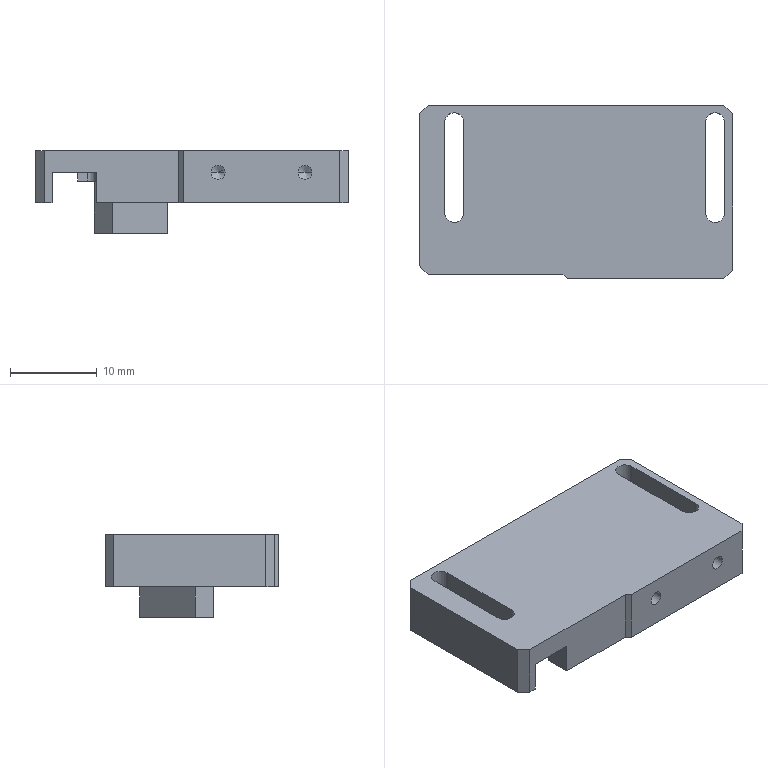Part | 1 solid | 54 faces | box 36 x 20 x 9.5 mm | volume 2604 mm3 | plane 35 | cylinder 15 | cone 4 | commonest cylinder face diameters 2.2 x6 2 x5 1.6 x4